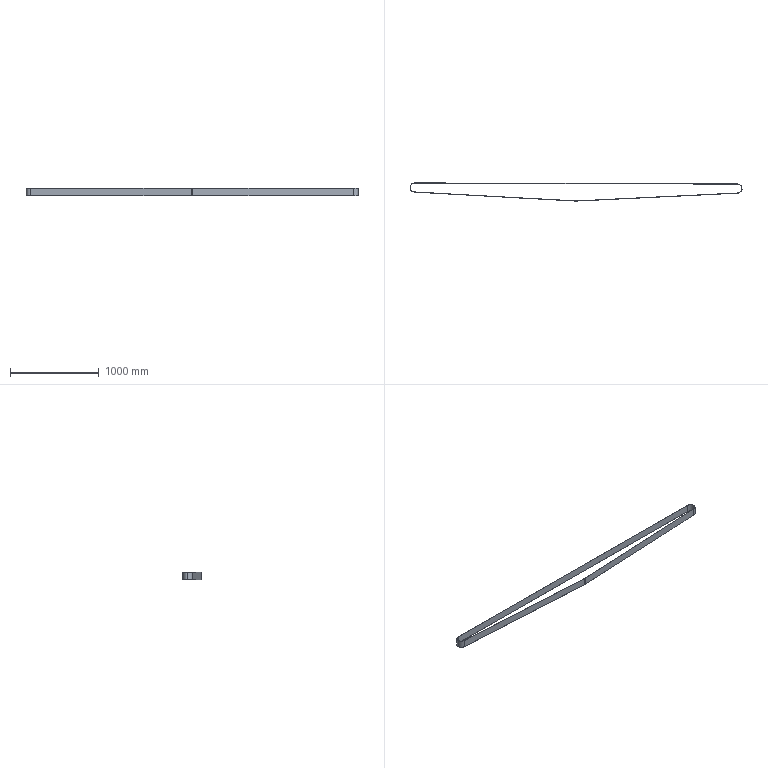Part | STEP file | T10 timing belt-1-2 | 1 solid | 16 faces | box 3744 x 205.239 x 85 mm | volume 1293096 mm3 | cylinder 8 | plane 8 | commonest cylinder face diameters 100 x3 104 x3 294.523 x1 298.523 x1
STEP:
#1=CARTESIAN_POINT('',(0.,0.,0.));
#2=DIRECTION('',(0.,0.,1.));
#3=DIRECTION('',(1.,0.,0.));
#4=AXIS2_PLACEMENT_3D('',#1,#2,#3);
#5=CARTESIAN_POINT('',(0.1605,50.,85.));
#6=VERTEX_POINT('',#5);
#7=CARTESIAN_POINT('',(0.1605,50.,0.));
#8=VERTEX_POINT('',#7);
#9=CARTESIAN_POINT('',(0.1605,50.,85.));
#10=DIRECTION('',(0.,0.,-1.));
#11=VECTOR('',#10,1.);
#12=LINE('',#9,#11);
#13=CARTESIAN_POINT('',(-0.003728,0.0001534,85.));
#14=DIRECTION('',(0.,0.,-1.));
#15=DIRECTION('',(-1.,0.,0.));
#16=AXIS2_PLACEMENT_3D('',#13,#14,#15);
#17=CYLINDRICAL_SURFACE('',#16,50.);
#18=CARTESIAN_POINT('',(1.574,0.));
#19=DIRECTION('',(0.,1.));
#20=VECTOR('',#19,1.);
#21=LINE('',#18,#20);
#22=(GEOMETRIC_REPRESENTATION_CONTEXT(2)PARAMETRIC_REPRESENTATION_CONTEXT()REPRESENTATION_CONTEXT('',''));
#23=DEFINITIONAL_REPRESENTATION('',(#21),#22);
#24=PCURVE('',#17,#23);
#25=CARTESIAN_POINT('',(0.1605,50.,85.));
#26=DIRECTION('',(-0.003284,-1.,0.));
#27=DIRECTION('',(1.,-0.003284,0.));
#28=AXIS2_PLACEMENT_3D('',#25,#26,#27);
#29=PLANE('',#28);
#30=CARTESIAN_POINT('',(0.,0.));
#31=DIRECTION('',(0.,-1.));
#32=VECTOR('',#31,1.);
#33=LINE('',#30,#32);
#34=(GEOMETRIC_REPRESENTATION_CONTEXT(2)PARAMETRIC_REPRESENTATION_CONTEXT()REPRESENTATION_CONTEXT('',''));
#35=DEFINITIONAL_REPRESENTATION('',(#33),#34);
#36=PCURVE('',#29,#35);
#37=SURFACE_CURVE('',#12,(#24,#36),.PCURVE_S1.);
#38=EDGE_CURVE('',#6,#8,#37,.T.);
#39=ORIENTED_EDGE('',*,*,#38,.T.);
#40=CARTESIAN_POINT('',(-50.004,0.0001534,0.));
#41=VERTEX_POINT('',#40);
#42=CARTESIAN_POINT('',(-0.003728,0.0001534,0.));
#43=DIRECTION('',(0.,0.,1.));
#44=DIRECTION('',(1.,0.,0.));
#45=AXIS2_PLACEMENT_3D('',#42,#43,#44);
#46=CIRCLE('',#45,50.);
#47=CARTESIAN_POINT('',(3.142,85.));
#48=DIRECTION('',(-1.,0.));
#49=VECTOR('',#48,1.);
#50=LINE('',#47,#49);
#51=(GEOMETRIC_REPRESENTATION_CONTEXT(2)PARAMETRIC_REPRESENTATION_CONTEXT()REPRESENTATION_CONTEXT('',''));
#52=DEFINITIONAL_REPRESENTATION('',(#50),#51);
#53=PCURVE('',#17,#52);
#54=CARTESIAN_POINT('',(-0.003728,0.0001534,0.));
#55=DIRECTION('',(0.,0.,1.));
#56=DIRECTION('',(1.,0.,0.));
#57=AXIS2_PLACEMENT_3D('',#54,#55,#56);
#58=PLANE('',#57);
#59=CARTESIAN_POINT('',(0.,0.));
#60=DIRECTION('',(1.,0.));
#61=AXIS2_PLACEMENT_2D('',#59,#60);
#62=CIRCLE('',#61,50.);
#63=(GEOMETRIC_REPRESENTATION_CONTEXT(2)PARAMETRIC_REPRESENTATION_CONTEXT()REPRESENTATION_CONTEXT('',''));
#64=DEFINITIONAL_REPRESENTATION('',(#62),#63);
#65=PCURVE('',#58,#64);
#66=SURFACE_CURVE('',#46,(#53,#65),.PCURVE_S1.);
#67=EDGE_CURVE('',#8,#41,#66,.T.);
#68=ORIENTED_EDGE('',*,*,#67,.T.);
#69=CARTESIAN_POINT('',(-50.004,0.0001534,85.));
#70=VERTEX_POINT('',#69);
#71=CARTESIAN_POINT('',(-50.004,0.0001534,85.));
#72=DIRECTION('',(0.,0.,-1.));
#73=VECTOR('',#72,1.);
#74=LINE('',#71,#73);
#75=CARTESIAN_POINT('',(0.,0.));
#76=DIRECTION('',(0.,1.));
#77=VECTOR('',#76,1.);
#78=LINE('',#75,#77);
#79=(GEOMETRIC_REPRESENTATION_CONTEXT(2)PARAMETRIC_REPRESENTATION_CONTEXT()REPRESENTATION_CONTEXT('',''));
#80=DEFINITIONAL_REPRESENTATION('',(#78),#79);
#81=PCURVE('',#17,#80);
#82=CARTESIAN_POINT('',(-0.003728,0.0001534,85.));
#83=DIRECTION('',(0.,0.,-1.));
#84=DIRECTION('',(-1.,0.,0.));
#85=AXIS2_PLACEMENT_3D('',#82,#83,#84);
#86=CYLINDRICAL_SURFACE('',#85,50.);
#87=CARTESIAN_POINT('',(6.283,0.));
#88=DIRECTION('',(0.,1.));
#89=VECTOR('',#88,1.);
#90=LINE('',#87,#89);
#91=(GEOMETRIC_REPRESENTATION_CONTEXT(2)PARAMETRIC_REPRESENTATION_CONTEXT()REPRESENTATION_CONTEXT('',''));
#92=DEFINITIONAL_REPRESENTATION('',(#90),#91);
#93=PCURVE('',#86,#92);
#94=SURFACE_CURVE('',#74,(#81,#93),.PCURVE_S1.);
#95=EDGE_CURVE('',#70,#41,#94,.T.);
#96=ORIENTED_EDGE('',*,*,#95,.F.);
#97=CARTESIAN_POINT('',(-0.003728,0.0001534,85.));
#98=DIRECTION('',(0.,0.,1.));
#99=DIRECTION('',(1.,0.,0.));
#100=AXIS2_PLACEMENT_3D('',#97,#98,#99);
#101=CIRCLE('',#100,50.);
#102=CARTESIAN_POINT('',(3.142,0.));
#103=DIRECTION('',(-1.,0.));
#104=VECTOR('',#103,1.);
#105=LINE('',#102,#104);
#106=(GEOMETRIC_REPRESENTATION_CONTEXT(2)PARAMETRIC_REPRESENTATION_CONTEXT()REPRESENTATION_CONTEXT('',''));
#107=DEFINITIONAL_REPRESENTATION('',(#105),#106);
#108=PCURVE('',#17,#107);
#109=CARTESIAN_POINT('',(-0.003728,0.0001534,85.));
#110=DIRECTION('',(0.,0.,1.));
#111=DIRECTION('',(1.,0.,0.));
#112=AXIS2_PLACEMENT_3D('',#109,#110,#111);
#113=PLANE('',#112);
#114=CARTESIAN_POINT('',(0.,0.));
#115=DIRECTION('',(1.,0.));
#116=AXIS2_PLACEMENT_2D('',#114,#115);
#117=CIRCLE('',#116,50.);
#118=(GEOMETRIC_REPRESENTATION_CONTEXT(2)PARAMETRIC_REPRESENTATION_CONTEXT()REPRESENTATION_CONTEXT('',''));
#119=DEFINITIONAL_REPRESENTATION('',(#117),#118);
#120=PCURVE('',#113,#119);
#121=SURFACE_CURVE('',#101,(#108,#120),.PCURVE_S1.);
#122=EDGE_CURVE('',#6,#70,#121,.T.);
#123=ORIENTED_EDGE('',*,*,#122,.F.);
#124=EDGE_LOOP('',(#39,#68,#96,#123));
#125=FACE_BOUND('',#124,.F.);
#126=ADVANCED_FACE('',(#125),#17,.F.);
#127=CARTESIAN_POINT('',(-52.004,0.0001534,85.));
#128=VERTEX_POINT('',#127);
#129=CARTESIAN_POINT('',(-2.896,-51.919,85.));
#130=VERTEX_POINT('',#129);
#131=CARTESIAN_POINT('',(-0.003728,0.0001534,85.));
#132=DIRECTION('',(0.,0.,1.));
#133=DIRECTION('',(1.,0.,0.));
#134=AXIS2_PLACEMENT_3D('',#131,#132,#133);
#135=CIRCLE('',#134,52.);
#136=CARTESIAN_POINT('',(-0.003728,0.0001534,85.));
#137=DIRECTION('',(0.,0.,-1.));
#138=DIRECTION('',(-1.,0.,0.));
#139=AXIS2_PLACEMENT_3D('',#136,#137,#138);
#140=CYLINDRICAL_SURFACE('',#139,52.);
#141=CARTESIAN_POINT('',(9.425,0.));
#142=DIRECTION('',(-1.,0.));
#143=VECTOR('',#142,1.);
#144=LINE('',#141,#143);
#145=(GEOMETRIC_REPRESENTATION_CONTEXT(2)PARAMETRIC_REPRESENTATION_CONTEXT()REPRESENTATION_CONTEXT('',''));
#146=DEFINITIONAL_REPRESENTATION('',(#144),#145);
#147=PCURVE('',#140,#146);
#148=CARTESIAN_POINT('',(0.,0.));
#149=DIRECTION('',(1.,0.));
#150=AXIS2_PLACEMENT_2D('',#148,#149);
#151=CIRCLE('',#150,52.);
#152=(GEOMETRIC_REPRESENTATION_CONTEXT(2)PARAMETRIC_REPRESENTATION_CONTEXT()REPRESENTATION_CONTEXT('',''));
#153=DEFINITIONAL_REPRESENTATION('',(#151),#152);
#154=PCURVE('',#113,#153);
#155=SURFACE_CURVE('',#135,(#147,#154),.PCURVE_S1.);
#156=EDGE_CURVE('',#128,#130,#155,.T.);
#157=ORIENTED_EDGE('',*,*,#156,.F.);
#158=CARTESIAN_POINT('',(-52.004,0.0001534,0.));
#159=VERTEX_POINT('',#158);
#160=CARTESIAN_POINT('',(-52.004,0.0001534,85.));
#161=DIRECTION('',(0.,0.,-1.));
#162=VECTOR('',#161,1.);
#163=LINE('',#160,#162);
#164=CARTESIAN_POINT('',(6.283,0.));
#165=DIRECTION('',(0.,1.));
#166=VECTOR('',#165,1.);
#167=LINE('',#164,#166);
#168=(GEOMETRIC_REPRESENTATION_CONTEXT(2)PARAMETRIC_REPRESENTATION_CONTEXT()REPRESENTATION_CONTEXT('',''));
#169=DEFINITIONAL_REPRESENTATION('',(#167),#168);
#170=PCURVE('',#140,#169);
#171=CARTESIAN_POINT('',(-0.003728,0.0001534,85.));
#172=DIRECTION('',(0.,0.,-1.));
#173=DIRECTION('',(-1.,0.,0.));
#174=AXIS2_PLACEMENT_3D('',#171,#172,#173);
#175=CYLINDRICAL_SURFACE('',#174,52.);
#176=CARTESIAN_POINT('',(0.,0.));
#177=DIRECTION('',(0.,1.));
#178=VECTOR('',#177,1.);
#179=LINE('',#176,#178);
#180=(GEOMETRIC_REPRESENTATION_CONTEXT(2)PARAMETRIC_REPRESENTATION_CONTEXT()REPRESENTATION_CONTEXT('',''));
#181=DEFINITIONAL_REPRESENTATION('',(#179),#180);
#182=PCURVE('',#175,#181);
#183=SURFACE_CURVE('',#163,(#170,#182),.PCURVE_S1.);
#184=EDGE_CURVE('',#128,#159,#183,.T.);
#185=ORIENTED_EDGE('',*,*,#184,.T.);
#186=CARTESIAN_POINT('',(-2.896,-51.919,0.));
#187=VERTEX_POINT('',#186);
#188=CARTESIAN_POINT('',(-0.003728,0.0001534,0.));
#189=DIRECTION('',(0.,0.,1.));
#190=DIRECTION('',(1.,0.,0.));
#191=AXIS2_PLACEMENT_3D('',#188,#189,#190);
#192=CIRCLE('',#191,52.);
#193=CARTESIAN_POINT('',(9.425,85.));
#194=DIRECTION('',(-1.,0.));
#195=VECTOR('',#194,1.);
#196=LINE('',#193,#195);
#197=(GEOMETRIC_REPRESENTATION_CONTEXT(2)PARAMETRIC_REPRESENTATION_CONTEXT()REPRESENTATION_CONTEXT('',''));
#198=DEFINITIONAL_REPRESENTATION('',(#196),#197);
#199=PCURVE('',#140,#198);
#200=CARTESIAN_POINT('',(0.,0.));
#201=DIRECTION('',(1.,0.));
#202=AXIS2_PLACEMENT_2D('',#200,#201);
#203=CIRCLE('',#202,52.);
#204=(GEOMETRIC_REPRESENTATION_CONTEXT(2)PARAMETRIC_REPRESENTATION_CONTEXT()REPRESENTATION_CONTEXT('',''));
#205=DEFINITIONAL_REPRESENTATION('',(#203),#204);
#206=PCURVE('',#58,#205);
#207=SURFACE_CURVE('',#192,(#199,#206),.PCURVE_S1.);
#208=EDGE_CURVE('',#159,#187,#207,.T.);
#209=ORIENTED_EDGE('',*,*,#208,.T.);
#210=CARTESIAN_POINT('',(-2.896,-51.919,85.));
#211=DIRECTION('',(0.,0.,-1.));
#212=VECTOR('',#211,1.);
#213=LINE('',#210,#212);
#214=CARTESIAN_POINT('',(4.768,0.));
#215=DIRECTION('',(0.,1.));
#216=VECTOR('',#215,1.);
#217=LINE('',#214,#216);
#218=(GEOMETRIC_REPRESENTATION_CONTEXT(2)PARAMETRIC_REPRESENTATION_CONTEXT()REPRESENTATION_CONTEXT('',''));
#219=DEFINITIONAL_REPRESENTATION('',(#217),#218);
#220=PCURVE('',#140,#219);
#221=CARTESIAN_POINT('',(-2.896,-51.919,85.));
#222=DIRECTION('',(0.05561,0.9985,0.));
#223=DIRECTION('',(-0.9985,0.05561,0.));
#224=AXIS2_PLACEMENT_3D('',#221,#222,#223);
#225=PLANE('',#224);
#226=CARTESIAN_POINT('',(0.,0.));
#227=DIRECTION('',(0.,-1.));
#228=VECTOR('',#227,1.);
#229=LINE('',#226,#228);
#230=(GEOMETRIC_REPRESENTATION_CONTEXT(2)PARAMETRIC_REPRESENTATION_CONTEXT()REPRESENTATION_CONTEXT('',''));
#231=DEFINITIONAL_REPRESENTATION('',(#229),#230);
#232=PCURVE('',#225,#231);
#233=SURFACE_CURVE('',#213,(#220,#232),.PCURVE_S1.);
#234=EDGE_CURVE('',#130,#187,#233,.T.);
#235=ORIENTED_EDGE('',*,*,#234,.F.);
#236=EDGE_LOOP('',(#157,#185,#209,#235));
#237=FACE_BOUND('',#236,.T.);
#238=ADVANCED_FACE('',(#237),#140,.T.);
#239=CARTESIAN_POINT('',(0.167,52.,85.));
#240=VERTEX_POINT('',#239);
#241=CARTESIAN_POINT('',(-0.003728,0.0001534,85.));
#242=DIRECTION('',(0.,0.,1.));
#243=DIRECTION('',(1.,0.,0.));
#244=AXIS2_PLACEMENT_3D('',#241,#242,#243);
#245=CIRCLE('',#244,52.);
#246=CARTESIAN_POINT('',(0.,0.));
#247=DIRECTION('',(1.,0.));
#248=AXIS2_PLACEMENT_2D('',#246,#247);
#249=CIRCLE('',#248,52.);
#250=(GEOMETRIC_REPRESENTATION_CONTEXT(2)PARAMETRIC_REPRESENTATION_CONTEXT()REPRESENTATION_CONTEXT('',''));
#251=DEFINITIONAL_REPRESENTATION('',(#249),#250);
#252=PCURVE('',#113,#251);
#253=CARTESIAN_POINT('',(3.142,0.));
#254=DIRECTION('',(-1.,0.));
#255=VECTOR('',#254,1.);
#256=LINE('',#253,#255);
#257=(GEOMETRIC_REPRESENTATION_CONTEXT(2)PARAMETRIC_REPRESENTATION_CONTEXT()REPRESENTATION_CONTEXT('',''));
#258=DEFINITIONAL_REPRESENTATION('',(#256),#257);
#259=PCURVE('',#175,#258);
#260=SURFACE_CURVE('',#245,(#252,#259),.PCURVE_S1.);
#261=EDGE_CURVE('',#240,#128,#260,.T.);
#262=ORIENTED_EDGE('',*,*,#261,.T.);
#263=ORIENTED_EDGE('',*,*,#156,.T.);
#264=CARTESIAN_POINT('',(1811.937,-153.008,85.));
#265=VERTEX_POINT('',#264);
#266=CARTESIAN_POINT('',(-2.896,-51.919,85.));
#267=DIRECTION('',(0.9985,-0.05561,0.));
#268=VECTOR('',#267,1.);
#269=LINE('',#266,#268);
#270=CARTESIAN_POINT('',(-2.892,-51.92));
#271=DIRECTION('',(0.9985,-0.05561));
#272=VECTOR('',#271,1.);
#273=LINE('',#270,#272);
#274=(GEOMETRIC_REPRESENTATION_CONTEXT(2)PARAMETRIC_REPRESENTATION_CONTEXT()REPRESENTATION_CONTEXT('',''));
#275=DEFINITIONAL_REPRESENTATION('',(#273),#274);
#276=PCURVE('',#113,#275);
#277=CARTESIAN_POINT('',(0.,0.));
#278=DIRECTION('',(-1.,0.));
#279=VECTOR('',#278,1.);
#280=LINE('',#277,#279);
#281=(GEOMETRIC_REPRESENTATION_CONTEXT(2)PARAMETRIC_REPRESENTATION_CONTEXT()REPRESENTATION_CONTEXT('',''));
#282=DEFINITIONAL_REPRESENTATION('',(#280),#281);
#283=PCURVE('',#225,#282);
#284=SURFACE_CURVE('',#269,(#276,#283),.PCURVE_S1.);
#285=EDGE_CURVE('',#130,#265,#284,.T.);
#286=ORIENTED_EDGE('',*,*,#285,.T.);
#287=CARTESIAN_POINT('',(1827.56,-153.059,85.));
#288=VERTEX_POINT('',#287);
#289=CARTESIAN_POINT('',(1820.238,-3.977,85.));
#290=DIRECTION('',(0.,0.,1.));
#291=DIRECTION('',(1.,0.,0.));
#292=AXIS2_PLACEMENT_3D('',#289,#290,#291);
#293=CIRCLE('',#292,149.262);
#294=CARTESIAN_POINT('',(1820.242,-3.977));
#295=DIRECTION('',(1.,0.));
#296=AXIS2_PLACEMENT_2D('',#294,#295);
#297=CIRCLE('',#296,149.262);
#298=(GEOMETRIC_REPRESENTATION_CONTEXT(2)PARAMETRIC_REPRESENTATION_CONTEXT()REPRESENTATION_CONTEXT('',''));
#299=DEFINITIONAL_REPRESENTATION('',(#297),#298);
#300=PCURVE('',#113,#299);
#301=CARTESIAN_POINT('',(1820.238,-3.977,85.));
#302=DIRECTION('',(0.,0.,-1.));
#303=DIRECTION('',(-1.,0.,0.));
#304=AXIS2_PLACEMENT_3D('',#301,#302,#303);
#305=CYLINDRICAL_SURFACE('',#304,149.262);
#306=CARTESIAN_POINT('',(9.425,0.));
#307=DIRECTION('',(-1.,0.));
#308=VECTOR('',#307,1.);
#309=LINE('',#306,#308);
#310=(GEOMETRIC_REPRESENTATION_CONTEXT(2)PARAMETRIC_REPRESENTATION_CONTEXT()REPRESENTATION_CONTEXT('',''));
#311=DEFINITIONAL_REPRESENTATION('',(#309),#310);
#312=PCURVE('',#305,#311);
#313=SURFACE_CURVE('',#293,(#300,#312),.PCURVE_S1.);
#314=EDGE_CURVE('',#265,#288,#313,.T.);
#315=ORIENTED_EDGE('',*,*,#314,.T.);
#316=CARTESIAN_POINT('',(3643.037,-63.892,85.));
#317=VERTEX_POINT('',#316);
#318=CARTESIAN_POINT('',(1827.56,-153.059,85.));
#319=DIRECTION('',(0.9988,0.04906,0.));
#320=VECTOR('',#319,1.);
#321=LINE('',#318,#320);
#322=CARTESIAN_POINT('',(1827.564,-153.059));
#323=DIRECTION('',(0.9988,0.04906));
#324=VECTOR('',#323,1.);
#325=LINE('',#322,#324);
#326=(GEOMETRIC_REPRESENTATION_CONTEXT(2)PARAMETRIC_REPRESENTATION_CONTEXT()REPRESENTATION_CONTEXT('',''));
#327=DEFINITIONAL_REPRESENTATION('',(#325),#326);
#328=PCURVE('',#113,#327);
#329=CARTESIAN_POINT('',(1827.56,-153.059,85.));
#330=DIRECTION('',(-0.04906,0.9988,0.));
#331=DIRECTION('',(-0.9988,-0.04906,0.));
#332=AXIS2_PLACEMENT_3D('',#329,#330,#331);
#333=PLANE('',#332);
#334=CARTESIAN_POINT('',(0.,0.));
#335=DIRECTION('',(-1.,0.));
#336=VECTOR('',#335,1.);
#337=LINE('',#334,#336);
#338=(GEOMETRIC_REPRESENTATION_CONTEXT(2)PARAMETRIC_REPRESENTATION_CONTEXT()REPRESENTATION_CONTEXT('',''));
#339=DEFINITIONAL_REPRESENTATION('',(#337),#338);
#340=PCURVE('',#333,#339);
#341=SURFACE_CURVE('',#321,(#328,#340),.PCURVE_S1.);
#342=EDGE_CURVE('',#288,#317,#341,.T.);
#343=ORIENTED_EDGE('',*,*,#342,.T.);
#344=CARTESIAN_POINT('',(3640.657,40.045,85.));
#345=VERTEX_POINT('',#344);
#346=CARTESIAN_POINT('',(3640.486,-11.955,85.));
#347=DIRECTION('',(0.,0.,1.));
#348=DIRECTION('',(-1.,0.,0.));
#349=AXIS2_PLACEMENT_3D('',#346,#347,#348);
#350=CIRCLE('',#349,52.);
#351=CARTESIAN_POINT('',(3640.49,-11.955));
#352=DIRECTION('',(-1.,0.));
#353=AXIS2_PLACEMENT_2D('',#351,#352);
#354=CIRCLE('',#353,52.);
#355=(GEOMETRIC_REPRESENTATION_CONTEXT(2)PARAMETRIC_REPRESENTATION_CONTEXT()REPRESENTATION_CONTEXT('',''));
#356=DEFINITIONAL_REPRESENTATION('',(#354),#355);
#357=PCURVE('',#113,#356);
#358=CARTESIAN_POINT('',(3640.486,-11.955,85.));
#359=DIRECTION('',(0.,0.,-1.));
#360=DIRECTION('',(-1.,0.,0.));
#361=AXIS2_PLACEMENT_3D('',#358,#359,#360);
#362=CYLINDRICAL_SURFACE('',#361,52.);
#363=CARTESIAN_POINT('',(6.283,0.));
#364=DIRECTION('',(-1.,0.));
#365=VECTOR('',#364,1.);
#366=LINE('',#363,#365);
#367=(GEOMETRIC_REPRESENTATION_CONTEXT(2)PARAMETRIC_REPRESENTATION_CONTEXT()REPRESENTATION_CONTEXT('',''));
#368=DEFINITIONAL_REPRESENTATION('',(#366),#367);
#369=PCURVE('',#362,#368);
#370=SURFACE_CURVE('',#350,(#357,#369),.PCURVE_S1.);
#371=EDGE_CURVE('',#317,#345,#370,.T.);
#372=ORIENTED_EDGE('',*,*,#371,.T.);
#373=CARTESIAN_POINT('',(0.167,52.,85.));
#374=DIRECTION('',(-1.,0.003284,0.));
#375=VECTOR('',#374,1.);
#376=LINE('',#373,#375);
#377=CARTESIAN_POINT('',(0.1708,52.));
#378=DIRECTION('',(-1.,0.003284));
#379=VECTOR('',#378,1.);
#380=LINE('',#377,#379);
#381=(GEOMETRIC_REPRESENTATION_CONTEXT(2)PARAMETRIC_REPRESENTATION_CONTEXT()REPRESENTATION_CONTEXT('',''));
#382=DEFINITIONAL_REPRESENTATION('',(#380),#381);
#383=PCURVE('',#113,#382);
#384=CARTESIAN_POINT('',(0.167,52.,85.));
#385=DIRECTION('',(-0.003284,-1.,0.));
#386=DIRECTION('',(1.,-0.003284,0.));
#387=AXIS2_PLACEMENT_3D('',#384,#385,#386);
#388=PLANE('',#387);
#389=CARTESIAN_POINT('',(0.,0.));
#390=DIRECTION('',(-1.,0.));
#391=VECTOR('',#390,1.);
#392=LINE('',#389,#391);
#393=(GEOMETRIC_REPRESENTATION_CONTEXT(2)PARAMETRIC_REPRESENTATION_CONTEXT()REPRESENTATION_CONTEXT('',''));
#394=DEFINITIONAL_REPRESENTATION('',(#392),#393);
#395=PCURVE('',#388,#394);
#396=SURFACE_CURVE('',#376,(#383,#395),.PCURVE_S1.);
#397=EDGE_CURVE('',#345,#240,#396,.T.);
#398=ORIENTED_EDGE('',*,*,#397,.T.);
#399=EDGE_LOOP('',(#262,#263,#286,#315,#343,#372,#398));
#400=FACE_BOUND('',#399,.T.);
#401=CARTESIAN_POINT('',(1827.462,-151.061,85.));
#402=VERTEX_POINT('',#401);
#403=CARTESIAN_POINT('',(3642.939,-61.894,85.));
#404=VERTEX_POINT('',#403);
#405=CARTESIAN_POINT('',(1827.462,-151.061,85.));
#406=DIRECTION('',(0.9988,0.04906,0.));
#407=VECTOR('',#406,1.);
#408=LINE('',#405,#407);
#409=CARTESIAN_POINT('',(1827.466,-151.062));
#410=DIRECTION('',(0.9988,0.04906));
#411=VECTOR('',#410,1.);
#412=LINE('',#409,#411);
#413=(GEOMETRIC_REPRESENTATION_CONTEXT(2)PARAMETRIC_REPRESENTATION_CONTEXT()REPRESENTATION_CONTEXT('',''));
#414=DEFINITIONAL_REPRESENTATION('',(#412),#413);
#415=PCURVE('',#113,#414);
#416=CARTESIAN_POINT('',(1827.462,-151.061,85.));
#417=DIRECTION('',(-0.04906,0.9988,0.));
#418=DIRECTION('',(-0.9988,-0.04906,0.));
#419=AXIS2_PLACEMENT_3D('',#416,#417,#418);
#420=PLANE('',#419);
#421=CARTESIAN_POINT('',(0.,0.));
#422=DIRECTION('',(-1.,0.));
#423=VECTOR('',#422,1.);
#424=LINE('',#421,#423);
#425=(GEOMETRIC_REPRESENTATION_CONTEXT(2)PARAMETRIC_REPRESENTATION_CONTEXT()REPRESENTATION_CONTEXT('',''));
#426=DEFINITIONAL_REPRESENTATION('',(#424),#425);
#427=PCURVE('',#420,#426);
#428=SURFACE_CURVE('',#408,(#415,#427),.PCURVE_S1.);
#429=EDGE_CURVE('',#402,#404,#428,.T.);
#430=ORIENTED_EDGE('',*,*,#429,.F.);
#431=CARTESIAN_POINT('',(1812.048,-151.011,85.));
#432=VERTEX_POINT('',#431);
#433=CARTESIAN_POINT('',(1820.238,-3.977,85.));
#434=DIRECTION('',(0.,0.,1.));
#435=DIRECTION('',(1.,0.,0.));
#436=AXIS2_PLACEMENT_3D('',#433,#434,#435);
#437=CIRCLE('',#436,147.262);
#438=CARTESIAN_POINT('',(1820.242,-3.977));
#439=DIRECTION('',(1.,0.));
#440=AXIS2_PLACEMENT_2D('',#438,#439);
#441=CIRCLE('',#440,147.262);
#442=(GEOMETRIC_REPRESENTATION_CONTEXT(2)PARAMETRIC_REPRESENTATION_CONTEXT()REPRESENTATION_CONTEXT('',''));
#443=DEFINITIONAL_REPRESENTATION('',(#441),#442);
#444=PCURVE('',#113,#443);
#445=CARTESIAN_POINT('',(1820.238,-3.977,85.));
#446=DIRECTION('',(0.,0.,-1.));
#447=DIRECTION('',(-1.,0.,0.));
#448=AXIS2_PLACEMENT_3D('',#445,#446,#447);
#449=CYLINDRICAL_SURFACE('',#448,147.262);
#450=CARTESIAN_POINT('',(9.425,0.));
#451=DIRECTION('',(-1.,0.));
#452=VECTOR('',#451,1.);
#453=LINE('',#450,#452);
#454=(GEOMETRIC_REPRESENTATION_CONTEXT(2)PARAMETRIC_REPRESENTATION_CONTEXT()REPRESENTATION_CONTEXT('',''));
#455=DEFINITIONAL_REPRESENTATION('',(#453),#454);
#456=PCURVE('',#449,#455);
#457=SURFACE_CURVE('',#437,(#444,#456),.PCURVE_S1.);
#458=EDGE_CURVE('',#432,#402,#457,.T.);
#459=ORIENTED_EDGE('',*,*,#458,.F.);
#460=CARTESIAN_POINT('',(-2.784,-49.922,85.));
#461=VERTEX_POINT('',#460);
#462=CARTESIAN_POINT('',(-2.784,-49.922,85.));
#463=DIRECTION('',(0.9985,-0.05561,0.));
#464=VECTOR('',#463,1.);
#465=LINE('',#462,#464);
#466=CARTESIAN_POINT('',(-2.781,-49.923));
#467=DIRECTION('',(0.9985,-0.05561));
#468=VECTOR('',#467,1.);
#469=LINE('',#466,#468);
#470=(GEOMETRIC_REPRESENTATION_CONTEXT(2)PARAMETRIC_REPRESENTATION_CONTEXT()REPRESENTATION_CONTEXT('',''));
#471=DEFINITIONAL_REPRESENTATION('',(#469),#470);
#472=PCURVE('',#113,#471);
#473=CARTESIAN_POINT('',(-2.784,-49.922,85.));
#474=DIRECTION('',(0.05561,0.9985,0.));
#475=DIRECTION('',(-0.9985,0.05561,0.));
#476=AXIS2_PLACEMENT_3D('',#473,#474,#475);
#477=PLANE('',#476);
#478=CARTESIAN_POINT('',(0.,0.));
#479=DIRECTION('',(-1.,0.));
#480=VECTOR('',#479,1.);
#481=LINE('',#478,#480);
#482=(GEOMETRIC_REPRESENTATION_CONTEXT(2)PARAMETRIC_REPRESENTATION_CONTEXT()REPRESENTATION_CONTEXT('',''));
#483=DEFINITIONAL_REPRESENTATION('',(#481),#482);
#484=PCURVE('',#477,#483);
#485=SURFACE_CURVE('',#465,(#472,#484),.PCURVE_S1.);
#486=EDGE_CURVE('',#461,#432,#485,.T.);
#487=ORIENTED_EDGE('',*,*,#486,.F.);
#488=CARTESIAN_POINT('',(-0.003728,0.0001534,85.));
#489=DIRECTION('',(0.,0.,1.));
#490=DIRECTION('',(1.,0.,0.));
#491=AXIS2_PLACEMENT_3D('',#488,#489,#490);
#492=CIRCLE('',#491,50.);
#493=CARTESIAN_POINT('',(0.,0.));
#494=DIRECTION('',(1.,0.));
#495=AXIS2_PLACEMENT_2D('',#493,#494);
#496=CIRCLE('',#495,50.);
#497=(GEOMETRIC_REPRESENTATION_CONTEXT(2)PARAMETRIC_REPRESENTATION_CONTEXT()REPRESENTATION_CONTEXT('',''));
#498=DEFINITIONAL_REPRESENTATION('',(#496),#497);
#499=PCURVE('',#113,#498);
#500=CARTESIAN_POINT('',(9.425,0.));
#501=DIRECTION('',(-1.,0.));
#502=VECTOR('',#501,1.);
#503=LINE('',#500,#502);
#504=(GEOMETRIC_REPRESENTATION_CONTEXT(2)PARAMETRIC_REPRESENTATION_CONTEXT()REPRESENTATION_CONTEXT('',''));
#505=DEFINITIONAL_REPRESENTATION('',(#503),#504);
#506=PCURVE('',#86,#505);
#507=SURFACE_CURVE('',#492,(#499,#506),.PCURVE_S1.);
#508=EDGE_CURVE('',#70,#461,#507,.T.);
#509=ORIENTED_EDGE('',*,*,#508,.F.);
#510=ORIENTED_EDGE('',*,*,#122,.F.);
#511=CARTESIAN_POINT('',(3640.65,38.045,85.));
#512=VERTEX_POINT('',#511);
#513=CARTESIAN_POINT('',(0.1605,50.,85.));
#514=DIRECTION('',(-1.,0.003284,0.));
#515=VECTOR('',#514,1.);
#516=LINE('',#513,#515);
#517=CARTESIAN_POINT('',(0.1642,50.));
#518=DIRECTION('',(-1.,0.003284));
#519=VECTOR('',#518,1.);
#520=LINE('',#517,#519);
#521=(GEOMETRIC_REPRESENTATION_CONTEXT(2)PARAMETRIC_REPRESENTATION_CONTEXT()REPRESENTATION_CONTEXT('',''));
#522=DEFINITIONAL_REPRESENTATION('',(#520),#521);
#523=PCURVE('',#113,#522);
#524=CARTESIAN_POINT('',(0.,0.));
#525=DIRECTION('',(-1.,0.));
#526=VECTOR('',#525,1.);
#527=LINE('',#524,#526);
#528=(GEOMETRIC_REPRESENTATION_CONTEXT(2)PARAMETRIC_REPRESENTATION_CONTEXT()REPRESENTATION_CONTEXT('',''));
#529=DEFINITIONAL_REPRESENTATION('',(#527),#528);
#530=PCURVE('',#29,#529);
#531=SURFACE_CURVE('',#516,(#523,#530),.PCURVE_S1.);
#532=EDGE_CURVE('',#512,#6,#531,.T.);
#533=ORIENTED_EDGE('',*,*,#532,.F.);
#534=CARTESIAN_POINT('',(3640.486,-11.955,85.));
#535=DIRECTION('',(0.,0.,1.));
#536=DIRECTION('',(-1.,0.,0.));
#537=AXIS2_PLACEMENT_3D('',#534,#535,#536);
#538=CIRCLE('',#537,50.);
#539=CARTESIAN_POINT('',(3640.49,-11.955));
#540=DIRECTION('',(-1.,0.));
#541=AXIS2_PLACEMENT_2D('',#539,#540);
#542=CIRCLE('',#541,50.);
#543=(GEOMETRIC_REPRESENTATION_CONTEXT(2)PARAMETRIC_REPRESENTATION_CONTEXT()REPRESENTATION_CONTEXT('',''));
#544=DEFINITIONAL_REPRESENTATION('',(#542),#543);
#545=PCURVE('',#113,#544);
#546=CARTESIAN_POINT('',(3640.486,-11.955,85.));
#547=DIRECTION('',(0.,0.,-1.));
#548=DIRECTION('',(-1.,0.,0.));
#549=AXIS2_PLACEMENT_3D('',#546,#547,#548);
#550=CYLINDRICAL_SURFACE('',#549,50.);
#551=CARTESIAN_POINT('',(6.283,0.));
#552=DIRECTION('',(-1.,0.));
#553=VECTOR('',#552,1.);
#554=LINE('',#551,#553);
#555=(GEOMETRIC_REPRESENTATION_CONTEXT(2)PARAMETRIC_REPRESENTATION_CONTEXT()REPRESENTATION_CONTEXT('',''));
#556=DEFINITIONAL_REPRESENTATION('',(#554),#555);
#557=PCURVE('',#550,#556);
#558=SURFACE_CURVE('',#538,(#545,#557),.PCURVE_S1.);
#559=EDGE_CURVE('',#404,#512,#558,.T.);
#560=ORIENTED_EDGE('',*,*,#559,.F.);
#561=EDGE_LOOP('',(#430,#459,#487,#509,#510,#533,#560));
#562=FACE_BOUND('',#561,.T.);
#563=ADVANCED_FACE('',(#400,#562),#113,.T.);
#564=CARTESIAN_POINT('',(0.167,52.,0.));
#565=VERTEX_POINT('',#564);
#566=CARTESIAN_POINT('',(-0.003728,0.0001534,0.));
#567=DIRECTION('',(0.,0.,1.));
#568=DIRECTION('',(1.,0.,0.));
#569=AXIS2_PLACEMENT_3D('',#566,#567,#568);
#570=CIRCLE('',#569,52.);
#571=CARTESIAN_POINT('',(0.,0.));
#572=DIRECTION('',(1.,0.));
#573=AXIS2_PLACEMENT_2D('',#571,#572);
#574=CIRCLE('',#573,52.);
#575=(GEOMETRIC_REPRESENTATION_CONTEXT(2)PARAMETRIC_REPRESENTATION_CONTEXT()REPRESENTATION_CONTEXT('',''));
#576=DEFINITIONAL_REPRESENTATION('',(#574),#575);
#577=PCURVE('',#58,#576);
#578=CARTESIAN_POINT('',(3.142,85.));
#579=DIRECTION('',(-1.,0.));
#580=VECTOR('',#579,1.);
#581=LINE('',#578,#580);
#582=(GEOMETRIC_REPRESENTATION_CONTEXT(2)PARAMETRIC_REPRESENTATION_CONTEXT()REPRESENTATION_CONTEXT('',''));
#583=DEFINITIONAL_REPRESENTATION('',(#581),#582);
#584=PCURVE('',#175,#583);
#585=SURFACE_CURVE('',#570,(#577,#584),.PCURVE_S1.);
#586=EDGE_CURVE('',#565,#159,#585,.T.);
#587=ORIENTED_EDGE('',*,*,#586,.F.);
#588=CARTESIAN_POINT('',(3640.657,40.045,0.));
#589=VERTEX_POINT('',#588);
#590=CARTESIAN_POINT('',(0.167,52.,0.));
#591=DIRECTION('',(-1.,0.003284,0.));
#592=VECTOR('',#591,1.);
#593=LINE('',#590,#592);
#594=CARTESIAN_POINT('',(0.1708,52.));
#595=DIRECTION('',(-1.,0.003284));
#596=VECTOR('',#595,1.);
#597=LINE('',#594,#596);
#598=(GEOMETRIC_REPRESENTATION_CONTEXT(2)PARAMETRIC_REPRESENTATION_CONTEXT()REPRESENTATION_CONTEXT('',''));
#599=DEFINITIONAL_REPRESENTATION('',(#597),#598);
#600=PCURVE('',#58,#599);
#601=CARTESIAN_POINT('',(0.,-85.));
#602=DIRECTION('',(-1.,0.));
#603=VECTOR('',#602,1.);
#604=LINE('',#601,#603);
#605=(GEOMETRIC_REPRESENTATION_CONTEXT(2)PARAMETRIC_REPRESENTATION_CONTEXT()REPRESENTATION_CONTEXT('',''));
#606=DEFINITIONAL_REPRESENTATION('',(#604),#605);
#607=PCURVE('',#388,#606);
#608=SURFACE_CURVE('',#593,(#600,#607),.PCURVE_S1.);
#609=EDGE_CURVE('',#589,#565,#608,.T.);
#610=ORIENTED_EDGE('',*,*,#609,.F.);
#611=CARTESIAN_POINT('',(3643.037,-63.892,0.));
#612=VERTEX_POINT('',#611);
#613=CARTESIAN_POINT('',(3640.486,-11.955,0.));
#614=DIRECTION('',(0.,0.,1.));
#615=DIRECTION('',(-1.,0.,0.));
#616=AXIS2_PLACEMENT_3D('',#613,#614,#615);
#617=CIRCLE('',#616,52.);
#618=CARTESIAN_POINT('',(3640.49,-11.955));
#619=DIRECTION('',(-1.,0.));
#620=AXIS2_PLACEMENT_2D('',#618,#619);
#621=CIRCLE('',#620,52.);
#622=(GEOMETRIC_REPRESENTATION_CONTEXT(2)PARAMETRIC_REPRESENTATION_CONTEXT()REPRESENTATION_CONTEXT('',''));
#623=DEFINITIONAL_REPRESENTATION('',(#621),#622);
#624=PCURVE('',#58,#623);
#625=CARTESIAN_POINT('',(6.283,85.));
#626=DIRECTION('',(-1.,0.));
#627=VECTOR('',#626,1.);
#628=LINE('',#625,#627);
#629=(GEOMETRIC_REPRESENTATION_CONTEXT(2)PARAMETRIC_REPRESENTATION_CONTEXT()REPRESENTATION_CONTEXT('',''));
#630=DEFINITIONAL_REPRESENTATION('',(#628),#629);
#631=PCURVE('',#362,#630);
#632=SURFACE_CURVE('',#617,(#624,#631),.PCURVE_S1.);
#633=EDGE_CURVE('',#612,#589,#632,.T.);
#634=ORIENTED_EDGE('',*,*,#633,.F.);
#635=CARTESIAN_POINT('',(1827.56,-153.059,0.));
#636=VERTEX_POINT('',#635);
#637=CARTESIAN_POINT('',(1827.56,-153.059,0.));
#638=DIRECTION('',(0.9988,0.04906,0.));
#639=VECTOR('',#638,1.);
#640=LINE('',#637,#639);
#641=CARTESIAN_POINT('',(1827.564,-153.059));
#642=DIRECTION('',(0.9988,0.04906));
#643=VECTOR('',#642,1.);
#644=LINE('',#641,#643);
#645=(GEOMETRIC_REPRESENTATION_CONTEXT(2)PARAMETRIC_REPRESENTATION_CONTEXT()REPRESENTATION_CONTEXT('',''));
#646=DEFINITIONAL_REPRESENTATION('',(#644),#645);
#647=PCURVE('',#58,#646);
#648=CARTESIAN_POINT('',(0.,-85.));
#649=DIRECTION('',(-1.,0.));
#650=VECTOR('',#649,1.);
#651=LINE('',#648,#650);
#652=(GEOMETRIC_REPRESENTATION_CONTEXT(2)PARAMETRIC_REPRESENTATION_CONTEXT()REPRESENTATION_CONTEXT('',''));
#653=DEFINITIONAL_REPRESENTATION('',(#651),#652);
#654=PCURVE('',#333,#653);
#655=SURFACE_CURVE('',#640,(#647,#654),.PCURVE_S1.);
#656=EDGE_CURVE('',#636,#612,#655,.T.);
#657=ORIENTED_EDGE('',*,*,#656,.F.);
#658=CARTESIAN_POINT('',(1811.937,-153.008,0.));
#659=VERTEX_POINT('',#658);
#660=CARTESIAN_POINT('',(1820.238,-3.977,0.));
#661=DIRECTION('',(0.,0.,1.));
#662=DIRECTION('',(1.,0.,0.));
#663=AXIS2_PLACEMENT_3D('',#660,#661,#662);
#664=CIRCLE('',#663,149.262);
#665=CARTESIAN_POINT('',(1820.242,-3.977));
#666=DIRECTION('',(1.,0.));
#667=AXIS2_PLACEMENT_2D('',#665,#666);
#668=CIRCLE('',#667,149.262);
#669=(GEOMETRIC_REPRESENTATION_CONTEXT(2)PARAMETRIC_REPRESENTATION_CONTEXT()REPRESENTATION_CONTEXT('',''));
#670=DEFINITIONAL_REPRESENTATION('',(#668),#669);
#671=PCURVE('',#58,#670);
#672=CARTESIAN_POINT('',(9.425,85.));
#673=DIRECTION('',(-1.,0.));
#674=VECTOR('',#673,1.);
#675=LINE('',#672,#674);
#676=(GEOMETRIC_REPRESENTATION_CONTEXT(2)PARAMETRIC_REPRESENTATION_CONTEXT()REPRESENTATION_CONTEXT('',''));
#677=DEFINITIONAL_REPRESENTATION('',(#675),#676);
#678=PCURVE('',#305,#677);
#679=SURFACE_CURVE('',#664,(#671,#678),.PCURVE_S1.);
#680=EDGE_CURVE('',#659,#636,#679,.T.);
#681=ORIENTED_EDGE('',*,*,#680,.F.);
#682=CARTESIAN_POINT('',(-2.896,-51.919,0.));
#683=DIRECTION('',(0.9985,-0.05561,0.));
#684=VECTOR('',#683,1.);
#685=LINE('',#682,#684);
#686=CARTESIAN_POINT('',(-2.892,-51.92));
#687=DIRECTION('',(0.9985,-0.05561));
#688=VECTOR('',#687,1.);
#689=LINE('',#686,#688);
#690=(GEOMETRIC_REPRESENTATION_CONTEXT(2)PARAMETRIC_REPRESENTATION_CONTEXT()REPRESENTATION_CONTEXT('',''));
#691=DEFINITIONAL_REPRESENTATION('',(#689),#690);
#692=PCURVE('',#58,#691);
#693=CARTESIAN_POINT('',(0.,-85.));
#694=DIRECTION('',(-1.,0.));
#695=VECTOR('',#694,1.);
#696=LINE('',#693,#695);
#697=(GEOMETRIC_REPRESENTATION_CONTEXT(2)PARAMETRIC_REPRESENTATION_CONTEXT()REPRESENTATION_CONTEXT('',''));
#698=DEFINITIONAL_REPRESENTATION('',(#696),#697);
#699=PCURVE('',#225,#698);
#700=SURFACE_CURVE('',#685,(#692,#699),.PCURVE_S1.);
#701=EDGE_CURVE('',#187,#659,#700,.T.);
#702=ORIENTED_EDGE('',*,*,#701,.F.);
#703=ORIENTED_EDGE('',*,*,#208,.F.);
#704=EDGE_LOOP('',(#587,#610,#634,#657,#681,#702,#703));
#705=FACE_BOUND('',#704,.T.);
#706=CARTESIAN_POINT('',(1812.048,-151.011,0.));
#707=VERTEX_POINT('',#706);
#708=CARTESIAN_POINT('',(1827.462,-151.061,0.));
#709=VERTEX_POINT('',#708);
#710=CARTESIAN_POINT('',(1820.238,-3.977,0.));
#711=DIRECTION('',(0.,0.,1.));
#712=DIRECTION('',(1.,0.,0.));
#713=AXIS2_PLACEMENT_3D('',#710,#711,#712);
#714=CIRCLE('',#713,147.262);
#715=CARTESIAN_POINT('',(1820.242,-3.977));
#716=DIRECTION('',(1.,0.));
#717=AXIS2_PLACEMENT_2D('',#715,#716);
#718=CIRCLE('',#717,147.262);
#719=(GEOMETRIC_REPRESENTATION_CONTEXT(2)PARAMETRIC_REPRESENTATION_CONTEXT()REPRESENTATION_CONTEXT('',''));
#720=DEFINITIONAL_REPRESENTATION('',(#718),#719);
#721=PCURVE('',#58,#720);
#722=CARTESIAN_POINT('',(9.425,85.));
#723=DIRECTION('',(-1.,0.));
#724=VECTOR('',#723,1.);
#725=LINE('',#722,#724);
#726=(GEOMETRIC_REPRESENTATION_CONTEXT(2)PARAMETRIC_REPRESENTATION_CONTEXT()REPRESENTATION_CONTEXT('',''));
#727=DEFINITIONAL_REPRESENTATION('',(#725),#726);
#728=PCURVE('',#449,#727);
#729=SURFACE_CURVE('',#714,(#721,#728),.PCURVE_S1.);
#730=EDGE_CURVE('',#707,#709,#729,.T.);
#731=ORIENTED_EDGE('',*,*,#730,.T.);
#732=CARTESIAN_POINT('',(3642.939,-61.894,0.));
#733=VERTEX_POINT('',#732);
#734=CARTESIAN_POINT('',(1827.462,-151.061,0.));
#735=DIRECTION('',(0.9988,0.04906,0.));
#736=VECTOR('',#735,1.);
#737=LINE('',#734,#736);
#738=CARTESIAN_POINT('',(1827.466,-151.062));
#739=DIRECTION('',(0.9988,0.04906));
#740=VECTOR('',#739,1.);
#741=LINE('',#738,#740);
#742=(GEOMETRIC_REPRESENTATION_CONTEXT(2)PARAMETRIC_REPRESENTATION_CONTEXT()REPRESENTATION_CONTEXT('',''));
#743=DEFINITIONAL_REPRESENTATION('',(#741),#742);
#744=PCURVE('',#58,#743);
#745=CARTESIAN_POINT('',(0.,-85.));
#746=DIRECTION('',(-1.,0.));
#747=VECTOR('',#746,1.);
#748=LINE('',#745,#747);
#749=(GEOMETRIC_REPRESENTATION_CONTEXT(2)PARAMETRIC_REPRESENTATION_CONTEXT()REPRESENTATION_CONTEXT('',''));
#750=DEFINITIONAL_REPRESENTATION('',(#748),#749);
#751=PCURVE('',#420,#750);
#752=SURFACE_CURVE('',#737,(#744,#751),.PCURVE_S1.);
#753=EDGE_CURVE('',#709,#733,#752,.T.);
#754=ORIENTED_EDGE('',*,*,#753,.T.);
#755=CARTESIAN_POINT('',(3640.65,38.045,0.));
#756=VERTEX_POINT('',#755);
#757=CARTESIAN_POINT('',(3640.486,-11.955,0.));
#758=DIRECTION('',(0.,0.,1.));
#759=DIRECTION('',(-1.,0.,0.));
#760=AXIS2_PLACEMENT_3D('',#757,#758,#759);
#761=CIRCLE('',#760,50.);
#762=CARTESIAN_POINT('',(3640.49,-11.955));
#763=DIRECTION('',(-1.,0.));
#764=AXIS2_PLACEMENT_2D('',#762,#763);
#765=CIRCLE('',#764,50.);
#766=(GEOMETRIC_REPRESENTATION_CONTEXT(2)PARAMETRIC_REPRESENTATION_CONTEXT()REPRESENTATION_CONTEXT('',''));
#767=DEFINITIONAL_REPRESENTATION('',(#765),#766);
#768=PCURVE('',#58,#767);
#769=CARTESIAN_POINT('',(6.283,85.));
#770=DIRECTION('',(-1.,0.));
#771=VECTOR('',#770,1.);
#772=LINE('',#769,#771);
#773=(GEOMETRIC_REPRESENTATION_CONTEXT(2)PARAMETRIC_REPRESENTATION_CONTEXT()REPRESENTATION_CONTEXT('',''));
#774=DEFINITIONAL_REPRESENTATION('',(#772),#773);
#775=PCURVE('',#550,#774);
#776=SURFACE_CURVE('',#761,(#768,#775),.PCURVE_S1.);
#777=EDGE_CURVE('',#733,#756,#776,.T.);
#778=ORIENTED_EDGE('',*,*,#777,.T.);
#779=CARTESIAN_POINT('',(0.1605,50.,0.));
#780=DIRECTION('',(-1.,0.003284,0.));
#781=VECTOR('',#780,1.);
#782=LINE('',#779,#781);
#783=CARTESIAN_POINT('',(0.1642,50.));
#784=DIRECTION('',(-1.,0.003284));
#785=VECTOR('',#784,1.);
#786=LINE('',#783,#785);
#787=(GEOMETRIC_REPRESENTATION_CONTEXT(2)PARAMETRIC_REPRESENTATION_CONTEXT()REPRESENTATION_CONTEXT('',''));
#788=DEFINITIONAL_REPRESENTATION('',(#786),#787);
#789=PCURVE('',#58,#788);
#790=CARTESIAN_POINT('',(0.,-85.));
#791=DIRECTION('',(-1.,0.));
#792=VECTOR('',#791,1.);
#793=LINE('',#790,#792);
#794=(GEOMETRIC_REPRESENTATION_CONTEXT(2)PARAMETRIC_REPRESENTATION_CONTEXT()REPRESENTATION_CONTEXT('',''));
#795=DEFINITIONAL_REPRESENTATION('',(#793),#794);
#796=PCURVE('',#29,#795);
#797=SURFACE_CURVE('',#782,(#789,#796),.PCURVE_S1.);
#798=EDGE_CURVE('',#756,#8,#797,.T.);
#799=ORIENTED_EDGE('',*,*,#798,.T.);
#800=ORIENTED_EDGE('',*,*,#67,.T.);
#801=CARTESIAN_POINT('',(-2.784,-49.922,0.));
#802=VERTEX_POINT('',#801);
#803=CARTESIAN_POINT('',(-0.003728,0.0001534,0.));
#804=DIRECTION('',(0.,0.,1.));
#805=DIRECTION('',(1.,0.,0.));
#806=AXIS2_PLACEMENT_3D('',#803,#804,#805);
#807=CIRCLE('',#806,50.);
#808=CARTESIAN_POINT('',(0.,0.));
#809=DIRECTION('',(1.,0.));
#810=AXIS2_PLACEMENT_2D('',#808,#809);
#811=CIRCLE('',#810,50.);
#812=(GEOMETRIC_REPRESENTATION_CONTEXT(2)PARAMETRIC_REPRESENTATION_CONTEXT()REPRESENTATION_CONTEXT('',''));
#813=DEFINITIONAL_REPRESENTATION('',(#811),#812);
#814=PCURVE('',#58,#813);
#815=CARTESIAN_POINT('',(9.425,85.));
#816=DIRECTION('',(-1.,0.));
#817=VECTOR('',#816,1.);
#818=LINE('',#815,#817);
#819=(GEOMETRIC_REPRESENTATION_CONTEXT(2)PARAMETRIC_REPRESENTATION_CONTEXT()REPRESENTATION_CONTEXT('',''));
#820=DEFINITIONAL_REPRESENTATION('',(#818),#819);
#821=PCURVE('',#86,#820);
#822=SURFACE_CURVE('',#807,(#814,#821),.PCURVE_S1.);
#823=EDGE_CURVE('',#41,#802,#822,.T.);
#824=ORIENTED_EDGE('',*,*,#823,.T.);
#825=CARTESIAN_POINT('',(-2.784,-49.922,0.));
#826=DIRECTION('',(0.9985,-0.05561,0.));
#827=VECTOR('',#826,1.);
#828=LINE('',#825,#827);
#829=CARTESIAN_POINT('',(-2.781,-49.923));
#830=DIRECTION('',(0.9985,-0.05561));
#831=VECTOR('',#830,1.);
#832=LINE('',#829,#831);
#833=(GEOMETRIC_REPRESENTATION_CONTEXT(2)PARAMETRIC_REPRESENTATION_CONTEXT()REPRESENTATION_CONTEXT('',''));
#834=DEFINITIONAL_REPRESENTATION('',(#832),#833);
#835=PCURVE('',#58,#834);
#836=CARTESIAN_POINT('',(0.,-85.));
#837=DIRECTION('',(-1.,0.));
#838=VECTOR('',#837,1.);
#839=LINE('',#836,#838);
#840=(GEOMETRIC_REPRESENTATION_CONTEXT(2)PARAMETRIC_REPRESENTATION_CONTEXT()REPRESENTATION_CONTEXT('',''));
#841=DEFINITIONAL_REPRESENTATION('',(#839),#840);
#842=PCURVE('',#477,#841);
#843=SURFACE_CURVE('',#828,(#835,#842),.PCURVE_S1.);
#844=EDGE_CURVE('',#802,#707,#843,.T.);
#845=ORIENTED_EDGE('',*,*,#844,.T.);
#846=EDGE_LOOP('',(#731,#754,#778,#799,#800,#824,#845));
#847=FACE_BOUND('',#846,.T.);
#848=ADVANCED_FACE('',(#705,#847),#58,.F.);
#849=ORIENTED_EDGE('',*,*,#184,.F.);
#850=ORIENTED_EDGE('',*,*,#261,.F.);
#851=CARTESIAN_POINT('',(0.167,52.,85.));
#852=DIRECTION('',(0.,0.,-1.));
#853=VECTOR('',#852,1.);
#854=LINE('',#851,#853);
#855=CARTESIAN_POINT('',(1.574,0.));
#856=DIRECTION('',(0.,1.));
#857=VECTOR('',#856,1.);
#858=LINE('',#855,#857);
#859=(GEOMETRIC_REPRESENTATION_CONTEXT(2)PARAMETRIC_REPRESENTATION_CONTEXT()REPRESENTATION_CONTEXT('',''));
#860=DEFINITIONAL_REPRESENTATION('',(#858),#859);
#861=PCURVE('',#175,#860);
#862=CARTESIAN_POINT('',(0.,0.));
#863=DIRECTION('',(0.,-1.));
#864=VECTOR('',#863,1.);
#865=LINE('',#862,#864);
#866=(GEOMETRIC_REPRESENTATION_CONTEXT(2)PARAMETRIC_REPRESENTATION_CONTEXT()REPRESENTATION_CONTEXT('',''));
#867=DEFINITIONAL_REPRESENTATION('',(#865),#866);
#868=PCURVE('',#388,#867);
#869=SURFACE_CURVE('',#854,(#861,#868),.PCURVE_S1.);
#870=EDGE_CURVE('',#240,#565,#869,.T.);
#871=ORIENTED_EDGE('',*,*,#870,.T.);
#872=ORIENTED_EDGE('',*,*,#586,.T.);
#873=EDGE_LOOP('',(#849,#850,#871,#872));
#874=FACE_BOUND('',#873,.T.);
#875=ADVANCED_FACE('',(#874),#175,.T.);
#876=ORIENTED_EDGE('',*,*,#701,.T.);
#877=CARTESIAN_POINT('',(1811.937,-153.008,85.));
#878=DIRECTION('',(0.,0.,-1.));
#879=VECTOR('',#878,1.);
#880=LINE('',#877,#879);
#881=CARTESIAN_POINT('',(-1817.646,0.));
#882=DIRECTION('',(0.,-1.));
#883=VECTOR('',#882,1.);
#884=LINE('',#881,#883);
#885=(GEOMETRIC_REPRESENTATION_CONTEXT(2)PARAMETRIC_REPRESENTATION_CONTEXT()REPRESENTATION_CONTEXT('',''));
#886=DEFINITIONAL_REPRESENTATION('',(#884),#885);
#887=PCURVE('',#225,#886);
#888=CARTESIAN_POINT('',(4.768,0.));
#889=DIRECTION('',(0.,1.));
#890=VECTOR('',#889,1.);
#891=LINE('',#888,#890);
#892=(GEOMETRIC_REPRESENTATION_CONTEXT(2)PARAMETRIC_REPRESENTATION_CONTEXT()REPRESENTATION_CONTEXT('',''));
#893=DEFINITIONAL_REPRESENTATION('',(#891),#892);
#894=PCURVE('',#305,#893);
#895=SURFACE_CURVE('',#880,(#887,#894),.PCURVE_S1.);
#896=EDGE_CURVE('',#265,#659,#895,.T.);
#897=ORIENTED_EDGE('',*,*,#896,.F.);
#898=ORIENTED_EDGE('',*,*,#285,.F.);
#899=ORIENTED_EDGE('',*,*,#234,.T.);
#900=EDGE_LOOP('',(#876,#897,#898,#899));
#901=FACE_BOUND('',#900,.T.);
#902=ADVANCED_FACE('',(#901),#225,.F.);
#903=ORIENTED_EDGE('',*,*,#680,.T.);
#904=CARTESIAN_POINT('',(1827.56,-153.059,85.));
#905=DIRECTION('',(0.,0.,-1.));
#906=VECTOR('',#905,1.);
#907=LINE('',#904,#906);
#908=CARTESIAN_POINT('',(4.663,0.));
#909=DIRECTION('',(0.,1.));
#910=VECTOR('',#909,1.);
#911=LINE('',#908,#910);
#912=(GEOMETRIC_REPRESENTATION_CONTEXT(2)PARAMETRIC_REPRESENTATION_CONTEXT()REPRESENTATION_CONTEXT('',''));
#913=DEFINITIONAL_REPRESENTATION('',(#911),#912);
#914=PCURVE('',#305,#913);
#915=CARTESIAN_POINT('',(0.,0.));
#916=DIRECTION('',(0.,-1.));
#917=VECTOR('',#916,1.);
#918=LINE('',#915,#917);
#919=(GEOMETRIC_REPRESENTATION_CONTEXT(2)PARAMETRIC_REPRESENTATION_CONTEXT()REPRESENTATION_CONTEXT('',''));
#920=DEFINITIONAL_REPRESENTATION('',(#918),#919);
#921=PCURVE('',#333,#920);
#922=SURFACE_CURVE('',#907,(#914,#921),.PCURVE_S1.);
#923=EDGE_CURVE('',#288,#636,#922,.T.);
#924=ORIENTED_EDGE('',*,*,#923,.F.);
#925=ORIENTED_EDGE('',*,*,#314,.F.);
#926=ORIENTED_EDGE('',*,*,#896,.T.);
#927=EDGE_LOOP('',(#903,#924,#925,#926));
#928=FACE_BOUND('',#927,.T.);
#929=ADVANCED_FACE('',(#928),#305,.T.);
#930=ORIENTED_EDGE('',*,*,#656,.T.);
#931=CARTESIAN_POINT('',(3643.037,-63.892,85.));
#932=DIRECTION('',(0.,0.,-1.));
#933=VECTOR('',#932,1.);
#934=LINE('',#931,#933);
#935=CARTESIAN_POINT('',(-1817.665,0.));
#936=DIRECTION('',(0.,-1.));
#937=VECTOR('',#936,1.);
#938=LINE('',#935,#937);
#939=(GEOMETRIC_REPRESENTATION_CONTEXT(2)PARAMETRIC_REPRESENTATION_CONTEXT()REPRESENTATION_CONTEXT('',''));
#940=DEFINITIONAL_REPRESENTATION('',(#938),#939);
#941=PCURVE('',#333,#940);
#942=CARTESIAN_POINT('',(4.663,0.));
#943=DIRECTION('',(0.,1.));
#944=VECTOR('',#943,1.);
#945=LINE('',#942,#944);
#946=(GEOMETRIC_REPRESENTATION_CONTEXT(2)PARAMETRIC_REPRESENTATION_CONTEXT()REPRESENTATION_CONTEXT('',''));
#947=DEFINITIONAL_REPRESENTATION('',(#945),#946);
#948=PCURVE('',#362,#947);
#949=SURFACE_CURVE('',#934,(#941,#948),.PCURVE_S1.);
#950=EDGE_CURVE('',#317,#612,#949,.T.);
#951=ORIENTED_EDGE('',*,*,#950,.F.);
#952=ORIENTED_EDGE('',*,*,#342,.F.);
#953=ORIENTED_EDGE('',*,*,#923,.T.);
#954=EDGE_LOOP('',(#930,#951,#952,#953));
#955=FACE_BOUND('',#954,.T.);
#956=ADVANCED_FACE('',(#955),#333,.F.);
#957=ORIENTED_EDGE('',*,*,#633,.T.);
#958=CARTESIAN_POINT('',(3640.657,40.045,85.));
#959=DIRECTION('',(0.,0.,-1.));
#960=VECTOR('',#959,1.);
#961=LINE('',#958,#960);
#962=CARTESIAN_POINT('',(1.574,0.));
#963=DIRECTION('',(0.,1.));
#964=VECTOR('',#963,1.);
#965=LINE('',#962,#964);
#966=(GEOMETRIC_REPRESENTATION_CONTEXT(2)PARAMETRIC_REPRESENTATION_CONTEXT()REPRESENTATION_CONTEXT('',''));
#967=DEFINITIONAL_REPRESENTATION('',(#965),#966);
#968=PCURVE('',#362,#967);
#969=CARTESIAN_POINT('',(3640.509,0.));
#970=DIRECTION('',(0.,-1.));
#971=VECTOR('',#970,1.);
#972=LINE('',#969,#971);
#973=(GEOMETRIC_REPRESENTATION_CONTEXT(2)PARAMETRIC_REPRESENTATION_CONTEXT()REPRESENTATION_CONTEXT('',''));
#974=DEFINITIONAL_REPRESENTATION('',(#972),#973);
#975=PCURVE('',#388,#974);
#976=SURFACE_CURVE('',#961,(#968,#975),.PCURVE_S1.);
#977=EDGE_CURVE('',#345,#589,#976,.T.);
#978=ORIENTED_EDGE('',*,*,#977,.F.);
#979=ORIENTED_EDGE('',*,*,#371,.F.);
#980=ORIENTED_EDGE('',*,*,#950,.T.);
#981=EDGE_LOOP('',(#957,#978,#979,#980));
#982=FACE_BOUND('',#981,.T.);
#983=ADVANCED_FACE('',(#982),#362,.T.);
#984=ORIENTED_EDGE('',*,*,#609,.T.);
#985=ORIENTED_EDGE('',*,*,#870,.F.);
#986=ORIENTED_EDGE('',*,*,#397,.F.);
#987=ORIENTED_EDGE('',*,*,#977,.T.);
#988=EDGE_LOOP('',(#984,#985,#986,#987));
#989=FACE_BOUND('',#988,.T.);
#990=ADVANCED_FACE('',(#989),#388,.F.);
#991=CARTESIAN_POINT('',(1827.462,-151.061,85.));
#992=DIRECTION('',(0.,0.,-1.));
#993=VECTOR('',#992,1.);
#994=LINE('',#991,#993);
#995=CARTESIAN_POINT('',(4.663,0.));
#996=DIRECTION('',(0.,1.));
#997=VECTOR('',#996,1.);
#998=LINE('',#995,#997);
#999=(GEOMETRIC_REPRESENTATION_CONTEXT(2)PARAMETRIC_REPRESENTATION_CONTEXT()REPRESENTATION_CONTEXT('',''));
#1000=DEFINITIONAL_REPRESENTATION('',(#998),#999);
#1001=PCURVE('',#449,#1000);
#1002=CARTESIAN_POINT('',(0.,0.));
#1003=DIRECTION('',(0.,-1.));
#1004=VECTOR('',#1003,1.);
#1005=LINE('',#1002,#1004);
#1006=(GEOMETRIC_REPRESENTATION_CONTEXT(2)PARAMETRIC_REPRESENTATION_CONTEXT()REPRESENTATION_CONTEXT('',''));
#1007=DEFINITIONAL_REPRESENTATION('',(#1005),#1006);
#1008=PCURVE('',#420,#1007);
#1009=SURFACE_CURVE('',#994,(#1001,#1008),.PCURVE_S1.);
#1010=EDGE_CURVE('',#402,#709,#1009,.T.);
#1011=ORIENTED_EDGE('',*,*,#1010,.F.);
#1012=ORIENTED_EDGE('',*,*,#458,.F.);
#1013=CARTESIAN_POINT('',(1812.048,-151.011,85.));
#1014=DIRECTION('',(0.,0.,-1.));
#1015=VECTOR('',#1014,1.);
#1016=LINE('',#1013,#1015);
#1017=CARTESIAN_POINT('',(4.768,0.));
#1018=DIRECTION('',(0.,1.));
#1019=VECTOR('',#1018,1.);
#1020=LINE('',#1017,#1019);
#1021=(GEOMETRIC_REPRESENTATION_CONTEXT(2)PARAMETRIC_REPRESENTATION_CONTEXT()REPRESENTATION_CONTEXT('',''));
#1022=DEFINITIONAL_REPRESENTATION('',(#1020),#1021);
#1023=PCURVE('',#449,#1022);
#1024=CARTESIAN_POINT('',(-1817.646,0.));
#1025=DIRECTION('',(0.,-1.));
#1026=VECTOR('',#1025,1.);
#1027=LINE('',#1024,#1026);
#1028=(GEOMETRIC_REPRESENTATION_CONTEXT(2)PARAMETRIC_REPRESENTATION_CONTEXT()REPRESENTATION_CONTEXT('',''));
#1029=DEFINITIONAL_REPRESENTATION('',(#1027),#1028);
#1030=PCURVE('',#477,#1029);
#1031=SURFACE_CURVE('',#1016,(#1023,#1030),.PCURVE_S1.);
#1032=EDGE_CURVE('',#432,#707,#1031,.T.);
#1033=ORIENTED_EDGE('',*,*,#1032,.T.);
#1034=ORIENTED_EDGE('',*,*,#730,.T.);
#1035=EDGE_LOOP('',(#1011,#1012,#1033,#1034));
#1036=FACE_BOUND('',#1035,.F.);
#1037=ADVANCED_FACE('',(#1036),#449,.F.);
#1038=ORIENTED_EDGE('',*,*,#753,.F.);
#1039=ORIENTED_EDGE('',*,*,#1010,.F.);
#1040=ORIENTED_EDGE('',*,*,#429,.T.);
#1041=CARTESIAN_POINT('',(3642.939,-61.894,85.));
#1042=DIRECTION('',(0.,0.,-1.));
#1043=VECTOR('',#1042,1.);
#1044=LINE('',#1041,#1043);
#1045=CARTESIAN_POINT('',(-1817.665,0.));
#1046=DIRECTION('',(0.,-1.));
#1047=VECTOR('',#1046,1.);
#1048=LINE('',#1045,#1047);
#1049=(GEOMETRIC_REPRESENTATION_CONTEXT(2)PARAMETRIC_REPRESENTATION_CONTEXT()REPRESENTATION_CONTEXT('',''));
#1050=DEFINITIONAL_REPRESENTATION('',(#1048),#1049);
#1051=PCURVE('',#420,#1050);
#1052=CARTESIAN_POINT('',(4.663,0.));
#1053=DIRECTION('',(0.,1.));
#1054=VECTOR('',#1053,1.);
#1055=LINE('',#1052,#1054);
#1056=(GEOMETRIC_REPRESENTATION_CONTEXT(2)PARAMETRIC_REPRESENTATION_CONTEXT()REPRESENTATION_CONTEXT('',''));
#1057=DEFINITIONAL_REPRESENTATION('',(#1055),#1056);
#1058=PCURVE('',#550,#1057);
#1059=SURFACE_CURVE('',#1044,(#1051,#1058),.PCURVE_S1.);
#1060=EDGE_CURVE('',#404,#733,#1059,.T.);
#1061=ORIENTED_EDGE('',*,*,#1060,.T.);
#1062=EDGE_LOOP('',(#1038,#1039,#1040,#1061));
#1063=FACE_BOUND('',#1062,.T.);
#1064=ADVANCED_FACE('',(#1063),#420,.T.);
#1065=CARTESIAN_POINT('',(3640.65,38.045,85.));
#1066=DIRECTION('',(0.,0.,-1.));
#1067=VECTOR('',#1066,1.);
#1068=LINE('',#1065,#1067);
#1069=CARTESIAN_POINT('',(1.574,0.));
#1070=DIRECTION('',(0.,1.));
#1071=VECTOR('',#1070,1.);
#1072=LINE('',#1069,#1071);
#1073=(GEOMETRIC_REPRESENTATION_CONTEXT(2)PARAMETRIC_REPRESENTATION_CONTEXT()REPRESENTATION_CONTEXT('',''));
#1074=DEFINITIONAL_REPRESENTATION('',(#1072),#1073);
#1075=PCURVE('',#550,#1074);
#1076=CARTESIAN_POINT('',(3640.509,0.));
#1077=DIRECTION('',(0.,-1.));
#1078=VECTOR('',#1077,1.);
#1079=LINE('',#1076,#1078);
#1080=(GEOMETRIC_REPRESENTATION_CONTEXT(2)PARAMETRIC_REPRESENTATION_CONTEXT()REPRESENTATION_CONTEXT('',''));
#1081=DEFINITIONAL_REPRESENTATION('',(#1079),#1080);
#1082=PCURVE('',#29,#1081);
#1083=SURFACE_CURVE('',#1068,(#1075,#1082),.PCURVE_S1.);
#1084=EDGE_CURVE('',#512,#756,#1083,.T.);
#1085=ORIENTED_EDGE('',*,*,#1084,.F.);
#1086=ORIENTED_EDGE('',*,*,#559,.F.);
#1087=ORIENTED_EDGE('',*,*,#1060,.T.);
#1088=ORIENTED_EDGE('',*,*,#777,.T.);
#1089=EDGE_LOOP('',(#1085,#1086,#1087,#1088));
#1090=FACE_BOUND('',#1089,.F.);
#1091=ADVANCED_FACE('',(#1090),#550,.F.);
#1092=ORIENTED_EDGE('',*,*,#798,.F.);
#1093=ORIENTED_EDGE('',*,*,#1084,.F.);
#1094=ORIENTED_EDGE('',*,*,#532,.T.);
#1095=ORIENTED_EDGE('',*,*,#38,.T.);
#1096=EDGE_LOOP('',(#1092,#1093,#1094,#1095));
#1097=FACE_BOUND('',#1096,.T.);
#1098=ADVANCED_FACE('',(#1097),#29,.T.);
#1099=ORIENTED_EDGE('',*,*,#823,.T.);
#1100=CARTESIAN_POINT('',(-2.784,-49.922,85.));
#1101=DIRECTION('',(0.,0.,-1.));
#1102=VECTOR('',#1101,1.);
#1103=LINE('',#1100,#1102);
#1104=CARTESIAN_POINT('',(4.768,0.));
#1105=DIRECTION('',(0.,1.));
#1106=VECTOR('',#1105,1.);
#1107=LINE('',#1104,#1106);
#1108=(GEOMETRIC_REPRESENTATION_CONTEXT(2)PARAMETRIC_REPRESENTATION_CONTEXT()REPRESENTATION_CONTEXT('',''));
#1109=DEFINITIONAL_REPRESENTATION('',(#1107),#1108);
#1110=PCURVE('',#86,#1109);
#1111=CARTESIAN_POINT('',(0.,0.));
#1112=DIRECTION('',(0.,-1.));
#1113=VECTOR('',#1112,1.);
#1114=LINE('',#1111,#1113);
#1115=(GEOMETRIC_REPRESENTATION_CONTEXT(2)PARAMETRIC_REPRESENTATION_CONTEXT()REPRESENTATION_CONTEXT('',''));
#1116=DEFINITIONAL_REPRESENTATION('',(#1114),#1115);
#1117=PCURVE('',#477,#1116);
#1118=SURFACE_CURVE('',#1103,(#1110,#1117),.PCURVE_S1.);
#1119=EDGE_CURVE('',#461,#802,#1118,.T.);
#1120=ORIENTED_EDGE('',*,*,#1119,.F.);
#1121=ORIENTED_EDGE('',*,*,#508,.F.);
#1122=ORIENTED_EDGE('',*,*,#95,.T.);
#1123=EDGE_LOOP('',(#1099,#1120,#1121,#1122));
#1124=FACE_BOUND('',#1123,.F.);
#1125=ADVANCED_FACE('',(#1124),#86,.F.);
#1126=ORIENTED_EDGE('',*,*,#844,.F.);
#1127=ORIENTED_EDGE('',*,*,#1119,.F.);
#1128=ORIENTED_EDGE('',*,*,#486,.T.);
#1129=ORIENTED_EDGE('',*,*,#1032,.T.);
#1130=EDGE_LOOP('',(#1126,#1127,#1128,#1129));
#1131=FACE_BOUND('',#1130,.T.);
#1132=ADVANCED_FACE('',(#1131),#477,.T.);
#1133=CLOSED_SHELL('',(#126,#238,#563,#848,#875,#902,#929,#956,#983,#990,#1037,#1064,#1091,#1098,#1125,#1132));
#1134=MANIFOLD_SOLID_BREP('',#1133);
#1135=(LENGTH_UNIT()NAMED_UNIT(*)SI_UNIT(.MILLI.,.METRE.));
#1136=UNCERTAINTY_MEASURE_WITH_UNIT(LENGTH_MEASURE(0.0000001),#1135,'','');
#1137=(NAMED_UNIT(*)PLANE_ANGLE_UNIT()SI_UNIT($,.RADIAN.));
#1138=(NAMED_UNIT(*)SI_UNIT($,.STERADIAN.)SOLID_ANGLE_UNIT());
#1139=(GEOMETRIC_REPRESENTATION_CONTEXT(3)GLOBAL_UNCERTAINTY_ASSIGNED_CONTEXT((#1136))GLOBAL_UNIT_ASSIGNED_CONTEXT((#1135,#1137,#1138))REPRESENTATION_CONTEXT('',''));
#1140=ADVANCED_BREP_SHAPE_REPRESENTATION('',(#4,#1134),#1139);